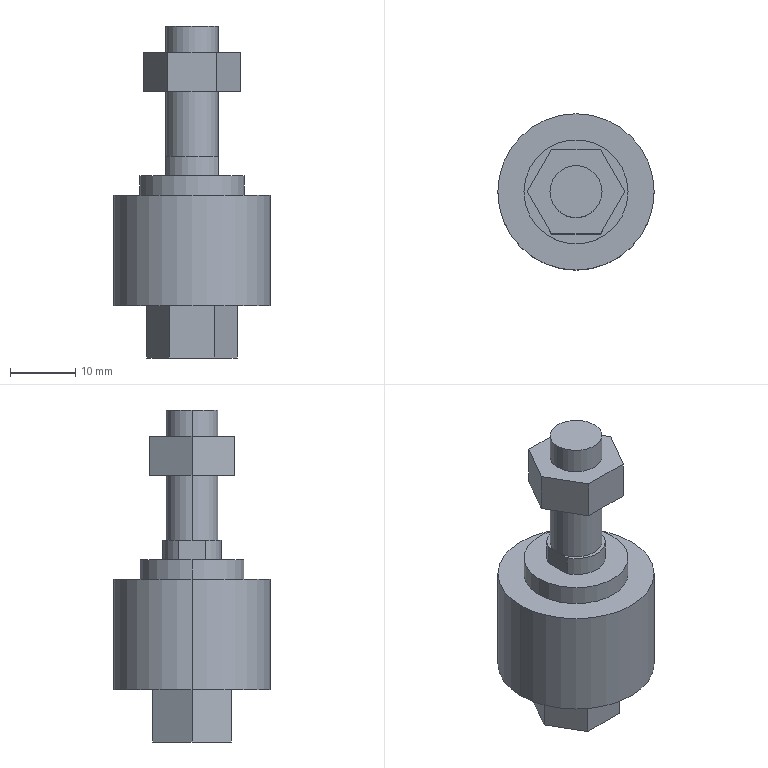Part | SolidWorks | features BaseBody 1 | 1 solid | 36 faces | box 24 x 24 x 51 mm | volume 10675 mm3 | plane 24 | cylinder 12 | commonest cylinder face diameters 8 x4 6.8 x2 9 x2 16 x2 24 x2
STEP:
#1=CARTESIAN_POINT('',(-3.4,0.,10.5));
#2=VERTEX_POINT('',#1);
#3=CARTESIAN_POINT('',(3.4,0.,10.5));
#4=VERTEX_POINT('',#3);
#5=CARTESIAN_POINT('',(0.,0.,10.5));
#6=DIRECTION('',(0.,0.,-1.));
#7=DIRECTION('',(-1.,0.,0.));
#8=AXIS2_PLACEMENT_3D('',#5,#6,#7);
#9=CIRCLE('',#8,3.4);
#10=EDGE_CURVE('',#2,#4,#9,.T.);
#11=ORIENTED_EDGE('',*,*,#10,.T.);
#12=CARTESIAN_POINT('',(0.,0.,10.5));
#13=DIRECTION('',(0.,0.,-1.));
#14=DIRECTION('',(-1.,0.,0.));
#15=AXIS2_PLACEMENT_3D('',#12,#13,#14);
#16=CIRCLE('',#15,3.4);
#17=EDGE_CURVE('',#4,#2,#16,.T.);
#18=ORIENTED_EDGE('',*,*,#17,.T.);
#19=EDGE_LOOP('',(#11,#18));
#20=FACE_OUTER_BOUND('',#19,.T.);
#21=CARTESIAN_POINT('',(0.,0.,10.5));
#22=DIRECTION('',(0.,0.,-1.));
#23=DIRECTION('',(0.,-1.,0.));
#24=AXIS2_PLACEMENT_3D('',#21,#22,#23);
#25=PLANE('',#24);
#26=ADVANCED_FACE('',(#20),#25,.T.);
#27=CARTESIAN_POINT('',(3.4,0.,0.));
#28=VERTEX_POINT('',#27);
#29=CARTESIAN_POINT('',(3.4,0.,10.5));
#30=DIRECTION('',(0.,0.,-1.));
#31=VECTOR('',#30,1000.);
#32=LINE('',#29,#31);
#33=EDGE_CURVE('',#4,#28,#32,.T.);
#34=ORIENTED_EDGE('',*,*,#33,.F.);
#35=ORIENTED_EDGE('',*,*,#10,.F.);
#36=CARTESIAN_POINT('',(-3.4,0.,0.));
#37=VERTEX_POINT('',#36);
#38=CARTESIAN_POINT('',(-3.4,0.,10.5));
#39=DIRECTION('',(0.,0.,-1.));
#40=VECTOR('',#39,1000.);
#41=LINE('',#38,#40);
#42=EDGE_CURVE('',#2,#37,#41,.T.);
#43=ORIENTED_EDGE('',*,*,#42,.T.);
#44=CARTESIAN_POINT('',(0.,0.,0.));
#45=DIRECTION('',(0.,0.,-1.));
#46=DIRECTION('',(-1.,0.,0.));
#47=AXIS2_PLACEMENT_3D('',#44,#45,#46);
#48=CIRCLE('',#47,3.4);
#49=EDGE_CURVE('',#37,#28,#48,.T.);
#50=ORIENTED_EDGE('',*,*,#49,.T.);
#51=EDGE_LOOP('',(#34,#35,#43,#50));
#52=FACE_OUTER_BOUND('',#51,.T.);
#53=CARTESIAN_POINT('',(0.,0.,10.5));
#54=DIRECTION('',(0.,0.,-1.));
#55=DIRECTION('',(-1.,0.,0.));
#56=AXIS2_PLACEMENT_3D('',#53,#54,#55);
#57=CYLINDRICAL_SURFACE('',#56,3.4);
#58=ADVANCED_FACE('',(#52),#57,.F.);
#59=CARTESIAN_POINT('',(4.,0.,51.));
#60=VERTEX_POINT('',#59);
#61=CARTESIAN_POINT('',(4.,0.,47.));
#62=VERTEX_POINT('',#61);
#63=CARTESIAN_POINT('',(4.,0.,0.));
#64=DIRECTION('',(0.,0.,-1.));
#65=VECTOR('',#64,1000.);
#66=LINE('',#63,#65);
#67=EDGE_CURVE('',#60,#62,#66,.T.);
#68=ORIENTED_EDGE('',*,*,#67,.F.);
#69=CARTESIAN_POINT('',(-4.,0.,51.));
#70=VERTEX_POINT('',#69);
#71=CARTESIAN_POINT('',(0.,0.,51.));
#72=DIRECTION('',(0.,0.,-1.));
#73=DIRECTION('',(-1.,0.,0.));
#74=AXIS2_PLACEMENT_3D('',#71,#72,#73);
#75=CIRCLE('',#74,4.);
#76=EDGE_CURVE('',#60,#70,#75,.T.);
#77=ORIENTED_EDGE('',*,*,#76,.T.);
#78=CARTESIAN_POINT('',(-4.,0.,47.));
#79=VERTEX_POINT('',#78);
#80=CARTESIAN_POINT('',(-4.,0.,0.));
#81=DIRECTION('',(0.,0.,-1.));
#82=VECTOR('',#81,1000.);
#83=LINE('',#80,#82);
#84=EDGE_CURVE('',#70,#79,#83,.T.);
#85=ORIENTED_EDGE('',*,*,#84,.T.);
#86=CARTESIAN_POINT('',(0.,0.,47.));
#87=DIRECTION('',(0.,0.,-1.));
#88=DIRECTION('',(1.,0.,0.));
#89=AXIS2_PLACEMENT_3D('',#86,#87,#88);
#90=CIRCLE('',#89,4.);
#91=EDGE_CURVE('',#62,#79,#90,.T.);
#92=ORIENTED_EDGE('',*,*,#91,.F.);
#93=EDGE_LOOP('',(#68,#77,#85,#92));
#94=FACE_OUTER_BOUND('',#93,.T.);
#95=CARTESIAN_POINT('',(0.,0.,0.));
#96=DIRECTION('',(0.,0.,-1.));
#97=DIRECTION('',(-1.,0.,0.));
#98=AXIS2_PLACEMENT_3D('',#95,#96,#97);
#99=CYLINDRICAL_SURFACE('',#98,4.);
#100=ADVANCED_FACE('',(#94),#99,.T.);
#101=CARTESIAN_POINT('',(0.,0.,51.));
#102=DIRECTION('',(0.,0.,-1.));
#103=DIRECTION('',(-1.,0.,0.));
#104=AXIS2_PLACEMENT_3D('',#101,#102,#103);
#105=CIRCLE('',#104,4.);
#106=EDGE_CURVE('',#70,#60,#105,.T.);
#107=ORIENTED_EDGE('',*,*,#106,.F.);
#108=ORIENTED_EDGE('',*,*,#76,.F.);
#109=EDGE_LOOP('',(#107,#108));
#110=FACE_OUTER_BOUND('',#109,.T.);
#111=CARTESIAN_POINT('',(0.,4.,51.));
#112=DIRECTION('',(0.,0.,1.));
#113=DIRECTION('',(1.,0.,0.));
#114=AXIS2_PLACEMENT_3D('',#111,#112,#113);
#115=PLANE('',#114);
#116=ADVANCED_FACE('',(#110),#115,.T.);
#117=CARTESIAN_POINT('',(0.,0.,47.));
#118=DIRECTION('',(0.,0.,-1.));
#119=DIRECTION('',(1.,0.,0.));
#120=AXIS2_PLACEMENT_3D('',#117,#118,#119);
#121=CIRCLE('',#120,4.);
#122=EDGE_CURVE('',#79,#62,#121,.T.);
#123=ORIENTED_EDGE('',*,*,#122,.T.);
#124=ORIENTED_EDGE('',*,*,#91,.T.);
#125=EDGE_LOOP('',(#123,#124));
#126=FACE_BOUND('',#125,.T.);
#127=CARTESIAN_POINT('',(-3.753,-6.5,47.));
#128=VERTEX_POINT('',#127);
#129=CARTESIAN_POINT('',(3.753,-6.5,47.));
#130=VERTEX_POINT('',#129);
#131=CARTESIAN_POINT('',(-3.753,-6.5,47.));
#132=DIRECTION('',(1.,0.,0.));
#133=VECTOR('',#132,1000.);
#134=LINE('',#131,#133);
#135=EDGE_CURVE('',#128,#130,#134,.T.);
#136=ORIENTED_EDGE('',*,*,#135,.T.);
#137=CARTESIAN_POINT('',(7.506,0.,47.));
#138=VERTEX_POINT('',#137);
#139=CARTESIAN_POINT('',(3.753,-6.5,47.));
#140=DIRECTION('',(0.5,0.866,0.));
#141=VECTOR('',#140,1000.);
#142=LINE('',#139,#141);
#143=EDGE_CURVE('',#130,#138,#142,.T.);
#144=ORIENTED_EDGE('',*,*,#143,.T.);
#145=CARTESIAN_POINT('',(3.753,6.5,47.));
#146=VERTEX_POINT('',#145);
#147=CARTESIAN_POINT('',(7.506,0.,47.));
#148=DIRECTION('',(-0.5,0.866,0.));
#149=VECTOR('',#148,1000.);
#150=LINE('',#147,#149);
#151=EDGE_CURVE('',#138,#146,#150,.T.);
#152=ORIENTED_EDGE('',*,*,#151,.T.);
#153=CARTESIAN_POINT('',(-3.753,6.5,47.));
#154=VERTEX_POINT('',#153);
#155=CARTESIAN_POINT('',(3.753,6.5,47.));
#156=DIRECTION('',(-1.,0.,0.));
#157=VECTOR('',#156,1000.);
#158=LINE('',#155,#157);
#159=EDGE_CURVE('',#146,#154,#158,.T.);
#160=ORIENTED_EDGE('',*,*,#159,.T.);
#161=CARTESIAN_POINT('',(-7.506,0.,47.));
#162=VERTEX_POINT('',#161);
#163=CARTESIAN_POINT('',(-3.753,6.5,47.));
#164=DIRECTION('',(-0.5,-0.866,0.));
#165=VECTOR('',#164,1000.);
#166=LINE('',#163,#165);
#167=EDGE_CURVE('',#154,#162,#166,.T.);
#168=ORIENTED_EDGE('',*,*,#167,.T.);
#169=CARTESIAN_POINT('',(-7.506,0.,47.));
#170=DIRECTION('',(0.5,-0.866,0.));
#171=VECTOR('',#170,1000.);
#172=LINE('',#169,#171);
#173=EDGE_CURVE('',#162,#128,#172,.T.);
#174=ORIENTED_EDGE('',*,*,#173,.T.);
#175=EDGE_LOOP('',(#136,#144,#152,#160,#168,#174));
#176=FACE_OUTER_BOUND('',#175,.T.);
#177=CARTESIAN_POINT('',(0.,0.,47.));
#178=DIRECTION('',(0.,0.,1.));
#179=DIRECTION('',(1.,0.,0.));
#180=AXIS2_PLACEMENT_3D('',#177,#178,#179);
#181=PLANE('',#180);
#182=ADVANCED_FACE('',(#126,#176),#181,.T.);
#183=CARTESIAN_POINT('',(-4.,0.,41.));
#184=VERTEX_POINT('',#183);
#185=CARTESIAN_POINT('',(4.,0.,41.));
#186=VERTEX_POINT('',#185);
#187=CARTESIAN_POINT('',(0.,0.,41.));
#188=DIRECTION('',(0.,0.,-1.));
#189=DIRECTION('',(1.,0.,0.));
#190=AXIS2_PLACEMENT_3D('',#187,#188,#189);
#191=CIRCLE('',#190,4.);
#192=EDGE_CURVE('',#184,#186,#191,.T.);
#193=ORIENTED_EDGE('',*,*,#192,.F.);
#194=CARTESIAN_POINT('',(0.,0.,41.));
#195=DIRECTION('',(0.,0.,-1.));
#196=DIRECTION('',(1.,0.,0.));
#197=AXIS2_PLACEMENT_3D('',#194,#195,#196);
#198=CIRCLE('',#197,4.);
#199=EDGE_CURVE('',#186,#184,#198,.T.);
#200=ORIENTED_EDGE('',*,*,#199,.F.);
#201=EDGE_LOOP('',(#193,#200));
#202=FACE_BOUND('',#201,.T.);
#203=CARTESIAN_POINT('',(-3.753,-6.5,41.));
#204=VERTEX_POINT('',#203);
#205=CARTESIAN_POINT('',(3.753,-6.5,41.));
#206=VERTEX_POINT('',#205);
#207=CARTESIAN_POINT('',(-3.753,-6.5,41.));
#208=DIRECTION('',(1.,0.,0.));
#209=VECTOR('',#208,1000.);
#210=LINE('',#207,#209);
#211=EDGE_CURVE('',#204,#206,#210,.T.);
#212=ORIENTED_EDGE('',*,*,#211,.F.);
#213=CARTESIAN_POINT('',(-7.506,0.,41.));
#214=VERTEX_POINT('',#213);
#215=CARTESIAN_POINT('',(-7.506,0.,41.));
#216=DIRECTION('',(0.5,-0.866,0.));
#217=VECTOR('',#216,1000.);
#218=LINE('',#215,#217);
#219=EDGE_CURVE('',#214,#204,#218,.T.);
#220=ORIENTED_EDGE('',*,*,#219,.F.);
#221=CARTESIAN_POINT('',(-3.753,6.5,41.));
#222=VERTEX_POINT('',#221);
#223=CARTESIAN_POINT('',(-3.753,6.5,41.));
#224=DIRECTION('',(-0.5,-0.866,0.));
#225=VECTOR('',#224,1000.);
#226=LINE('',#223,#225);
#227=EDGE_CURVE('',#222,#214,#226,.T.);
#228=ORIENTED_EDGE('',*,*,#227,.F.);
#229=CARTESIAN_POINT('',(3.753,6.5,41.));
#230=VERTEX_POINT('',#229);
#231=CARTESIAN_POINT('',(3.753,6.5,41.));
#232=DIRECTION('',(-1.,0.,0.));
#233=VECTOR('',#232,1000.);
#234=LINE('',#231,#233);
#235=EDGE_CURVE('',#230,#222,#234,.T.);
#236=ORIENTED_EDGE('',*,*,#235,.F.);
#237=CARTESIAN_POINT('',(7.506,0.,41.));
#238=VERTEX_POINT('',#237);
#239=CARTESIAN_POINT('',(7.506,0.,41.));
#240=DIRECTION('',(-0.5,0.866,0.));
#241=VECTOR('',#240,1000.);
#242=LINE('',#239,#241);
#243=EDGE_CURVE('',#238,#230,#242,.T.);
#244=ORIENTED_EDGE('',*,*,#243,.F.);
#245=CARTESIAN_POINT('',(3.753,-6.5,41.));
#246=DIRECTION('',(0.5,0.866,0.));
#247=VECTOR('',#246,1000.);
#248=LINE('',#245,#247);
#249=EDGE_CURVE('',#206,#238,#248,.T.);
#250=ORIENTED_EDGE('',*,*,#249,.F.);
#251=EDGE_LOOP('',(#212,#220,#228,#236,#244,#250));
#252=FACE_OUTER_BOUND('',#251,.T.);
#253=CARTESIAN_POINT('',(0.,0.,41.));
#254=DIRECTION('',(0.,0.,1.));
#255=DIRECTION('',(1.,0.,0.));
#256=AXIS2_PLACEMENT_3D('',#253,#254,#255);
#257=PLANE('',#256);
#258=ADVANCED_FACE('',(#202,#252),#257,.F.);
#259=ORIENTED_EDGE('',*,*,#143,.F.);
#260=CARTESIAN_POINT('',(3.753,-6.5,41.));
#261=DIRECTION('',(0.,0.,1.));
#262=VECTOR('',#261,1000.);
#263=LINE('',#260,#262);
#264=EDGE_CURVE('',#206,#130,#263,.T.);
#265=ORIENTED_EDGE('',*,*,#264,.F.);
#266=ORIENTED_EDGE('',*,*,#249,.T.);
#267=CARTESIAN_POINT('',(7.506,0.,41.));
#268=DIRECTION('',(0.,0.,1.));
#269=VECTOR('',#268,1000.);
#270=LINE('',#267,#269);
#271=EDGE_CURVE('',#238,#138,#270,.T.);
#272=ORIENTED_EDGE('',*,*,#271,.T.);
#273=EDGE_LOOP('',(#259,#265,#266,#272));
#274=FACE_OUTER_BOUND('',#273,.T.);
#275=CARTESIAN_POINT('',(3.753,-6.5,41.));
#276=DIRECTION('',(0.866,-0.5,0.));
#277=DIRECTION('',(0.,0.,-1.));
#278=AXIS2_PLACEMENT_3D('',#275,#276,#277);
#279=PLANE('',#278);
#280=ADVANCED_FACE('',(#274),#279,.T.);
#281=ORIENTED_EDGE('',*,*,#151,.F.);
#282=ORIENTED_EDGE('',*,*,#271,.F.);
#283=ORIENTED_EDGE('',*,*,#243,.T.);
#284=CARTESIAN_POINT('',(3.753,6.5,41.));
#285=DIRECTION('',(0.,0.,1.));
#286=VECTOR('',#285,1000.);
#287=LINE('',#284,#286);
#288=EDGE_CURVE('',#230,#146,#287,.T.);
#289=ORIENTED_EDGE('',*,*,#288,.T.);
#290=EDGE_LOOP('',(#281,#282,#283,#289));
#291=FACE_OUTER_BOUND('',#290,.T.);
#292=CARTESIAN_POINT('',(7.506,0.,41.));
#293=DIRECTION('',(0.866,0.5,0.));
#294=DIRECTION('',(0.,0.,-1.));
#295=AXIS2_PLACEMENT_3D('',#292,#293,#294);
#296=PLANE('',#295);
#297=ADVANCED_FACE('',(#291),#296,.T.);
#298=ORIENTED_EDGE('',*,*,#159,.F.);
#299=ORIENTED_EDGE('',*,*,#288,.F.);
#300=ORIENTED_EDGE('',*,*,#235,.T.);
#301=CARTESIAN_POINT('',(-3.753,6.5,41.));
#302=DIRECTION('',(0.,0.,1.));
#303=VECTOR('',#302,1000.);
#304=LINE('',#301,#303);
#305=EDGE_CURVE('',#222,#154,#304,.T.);
#306=ORIENTED_EDGE('',*,*,#305,.T.);
#307=EDGE_LOOP('',(#298,#299,#300,#306));
#308=FACE_OUTER_BOUND('',#307,.T.);
#309=CARTESIAN_POINT('',(3.753,6.5,41.));
#310=DIRECTION('',(0.,1.,0.));
#311=DIRECTION('',(1.,0.,0.));
#312=AXIS2_PLACEMENT_3D('',#309,#310,#311);
#313=PLANE('',#312);
#314=ADVANCED_FACE('',(#308),#313,.T.);
#315=ORIENTED_EDGE('',*,*,#167,.F.);
#316=ORIENTED_EDGE('',*,*,#305,.F.);
#317=ORIENTED_EDGE('',*,*,#227,.T.);
#318=CARTESIAN_POINT('',(-7.506,0.,41.));
#319=DIRECTION('',(0.,0.,1.));
#320=VECTOR('',#319,1000.);
#321=LINE('',#318,#320);
#322=EDGE_CURVE('',#214,#162,#321,.T.);
#323=ORIENTED_EDGE('',*,*,#322,.T.);
#324=EDGE_LOOP('',(#315,#316,#317,#323));
#325=FACE_OUTER_BOUND('',#324,.T.);
#326=CARTESIAN_POINT('',(-3.753,6.5,41.));
#327=DIRECTION('',(-0.866,0.5,0.));
#328=DIRECTION('',(0.,0.,1.));
#329=AXIS2_PLACEMENT_3D('',#326,#327,#328);
#330=PLANE('',#329);
#331=ADVANCED_FACE('',(#325),#330,.T.);
#332=ORIENTED_EDGE('',*,*,#173,.F.);
#333=ORIENTED_EDGE('',*,*,#322,.F.);
#334=ORIENTED_EDGE('',*,*,#219,.T.);
#335=CARTESIAN_POINT('',(-3.753,-6.5,41.));
#336=DIRECTION('',(0.,0.,1.));
#337=VECTOR('',#336,1000.);
#338=LINE('',#335,#337);
#339=EDGE_CURVE('',#204,#128,#338,.T.);
#340=ORIENTED_EDGE('',*,*,#339,.T.);
#341=EDGE_LOOP('',(#332,#333,#334,#340));
#342=FACE_OUTER_BOUND('',#341,.T.);
#343=CARTESIAN_POINT('',(-7.506,0.,41.));
#344=DIRECTION('',(-0.866,-0.5,0.));
#345=DIRECTION('',(-0.5,0.866,0.));
#346=AXIS2_PLACEMENT_3D('',#343,#344,#345);
#347=PLANE('',#346);
#348=ADVANCED_FACE('',(#342),#347,.T.);
#349=ORIENTED_EDGE('',*,*,#135,.F.);
#350=ORIENTED_EDGE('',*,*,#339,.F.);
#351=ORIENTED_EDGE('',*,*,#211,.T.);
#352=ORIENTED_EDGE('',*,*,#264,.T.);
#353=EDGE_LOOP('',(#349,#350,#351,#352));
#354=FACE_OUTER_BOUND('',#353,.T.);
#355=CARTESIAN_POINT('',(-3.753,-6.5,41.));
#356=DIRECTION('',(0.,-1.,0.));
#357=DIRECTION('',(0.,0.,-1.));
#358=AXIS2_PLACEMENT_3D('',#355,#356,#357);
#359=PLANE('',#358);
#360=ADVANCED_FACE('',(#354),#359,.T.);
#361=CARTESIAN_POINT('',(-4.,-2.062,28.));
#362=VERTEX_POINT('',#361);
#363=CARTESIAN_POINT('',(-4.,2.062,28.));
#364=VERTEX_POINT('',#363);
#365=CARTESIAN_POINT('',(-4.,-4.5,28.));
#366=DIRECTION('',(0.,1.,0.));
#367=VECTOR('',#366,1000.);
#368=LINE('',#365,#367);
#369=EDGE_CURVE('',#362,#364,#368,.T.);
#370=ORIENTED_EDGE('',*,*,#369,.F.);
#371=CARTESIAN_POINT('',(-4.,-2.062,31.));
#372=VERTEX_POINT('',#371);
#373=CARTESIAN_POINT('',(-4.,-2.062,0.));
#374=DIRECTION('',(0.,0.,-1.));
#375=VECTOR('',#374,1000.);
#376=LINE('',#373,#375);
#377=EDGE_CURVE('',#372,#362,#376,.T.);
#378=ORIENTED_EDGE('',*,*,#377,.F.);
#379=CARTESIAN_POINT('',(-4.,0.,31.));
#380=VERTEX_POINT('',#379);
#381=CARTESIAN_POINT('',(-4.,-4.5,31.));
#382=DIRECTION('',(0.,-1.,0.));
#383=VECTOR('',#382,1000.);
#384=LINE('',#381,#383);
#385=EDGE_CURVE('',#380,#372,#384,.T.);
#386=ORIENTED_EDGE('',*,*,#385,.F.);
#387=CARTESIAN_POINT('',(-4.,2.062,31.));
#388=VERTEX_POINT('',#387);
#389=CARTESIAN_POINT('',(-4.,-4.5,31.));
#390=DIRECTION('',(0.,-1.,0.));
#391=VECTOR('',#390,1000.);
#392=LINE('',#389,#391);
#393=EDGE_CURVE('',#388,#380,#392,.T.);
#394=ORIENTED_EDGE('',*,*,#393,.F.);
#395=CARTESIAN_POINT('',(-4.,2.062,0.));
#396=DIRECTION('',(0.,0.,1.));
#397=VECTOR('',#396,1000.);
#398=LINE('',#395,#397);
#399=EDGE_CURVE('',#364,#388,#398,.T.);
#400=ORIENTED_EDGE('',*,*,#399,.F.);
#401=EDGE_LOOP('',(#370,#378,#386,#394,#400));
#402=FACE_OUTER_BOUND('',#401,.T.);
#403=CARTESIAN_POINT('',(-4.,-4.5,-6.281));
#404=DIRECTION('',(-1.,0.,0.));
#405=DIRECTION('',(0.,0.,1.));
#406=AXIS2_PLACEMENT_3D('',#403,#404,#405);
#407=PLANE('',#406);
#408=ADVANCED_FACE('',(#402),#407,.T.);
#409=CARTESIAN_POINT('',(4.,2.062,28.));
#410=VERTEX_POINT('',#409);
#411=CARTESIAN_POINT('',(4.,-2.062,28.));
#412=VERTEX_POINT('',#411);
#413=CARTESIAN_POINT('',(4.,-4.5,28.));
#414=DIRECTION('',(0.,-1.,0.));
#415=VECTOR('',#414,1000.);
#416=LINE('',#413,#415);
#417=EDGE_CURVE('',#410,#412,#416,.T.);
#418=ORIENTED_EDGE('',*,*,#417,.F.);
#419=CARTESIAN_POINT('',(4.,2.062,31.));
#420=VERTEX_POINT('',#419);
#421=CARTESIAN_POINT('',(4.,2.062,0.));
#422=DIRECTION('',(0.,0.,-1.));
#423=VECTOR('',#422,1000.);
#424=LINE('',#421,#423);
#425=EDGE_CURVE('',#420,#410,#424,.T.);
#426=ORIENTED_EDGE('',*,*,#425,.F.);
#427=CARTESIAN_POINT('',(4.,0.,31.));
#428=VERTEX_POINT('',#427);
#429=CARTESIAN_POINT('',(4.,-4.5,31.));
#430=DIRECTION('',(0.,1.,0.));
#431=VECTOR('',#430,1000.);
#432=LINE('',#429,#431);
#433=EDGE_CURVE('',#428,#420,#432,.T.);
#434=ORIENTED_EDGE('',*,*,#433,.F.);
#435=CARTESIAN_POINT('',(4.,-2.062,31.));
#436=VERTEX_POINT('',#435);
#437=CARTESIAN_POINT('',(4.,-4.5,31.));
#438=DIRECTION('',(0.,1.,0.));
#439=VECTOR('',#438,1000.);
#440=LINE('',#437,#439);
#441=EDGE_CURVE('',#436,#428,#440,.T.);
#442=ORIENTED_EDGE('',*,*,#441,.F.);
#443=CARTESIAN_POINT('',(4.,-2.062,0.));
#444=DIRECTION('',(0.,0.,1.));
#445=VECTOR('',#444,1000.);
#446=LINE('',#443,#445);
#447=EDGE_CURVE('',#412,#436,#446,.T.);
#448=ORIENTED_EDGE('',*,*,#447,.F.);
#449=EDGE_LOOP('',(#418,#426,#434,#442,#448));
#450=FACE_OUTER_BOUND('',#449,.T.);
#451=CARTESIAN_POINT('',(4.,-4.5,-6.281));
#452=DIRECTION('',(1.,0.,0.));
#453=DIRECTION('',(0.,1.,0.));
#454=AXIS2_PLACEMENT_3D('',#451,#452,#453);
#455=PLANE('',#454);
#456=ADVANCED_FACE('',(#450),#455,.T.);
#457=CARTESIAN_POINT('',(0.,0.,28.));
#458=DIRECTION('',(0.,0.,-1.));
#459=DIRECTION('',(-1.,0.,0.));
#460=AXIS2_PLACEMENT_3D('',#457,#458,#459);
#461=CIRCLE('',#460,4.5);
#462=EDGE_CURVE('',#364,#410,#461,.T.);
#463=ORIENTED_EDGE('',*,*,#462,.T.);
#464=ORIENTED_EDGE('',*,*,#417,.T.);
#465=CARTESIAN_POINT('',(0.,0.,28.));
#466=DIRECTION('',(0.,0.,-1.));
#467=DIRECTION('',(-1.,0.,0.));
#468=AXIS2_PLACEMENT_3D('',#465,#466,#467);
#469=CIRCLE('',#468,4.5);
#470=EDGE_CURVE('',#412,#362,#469,.T.);
#471=ORIENTED_EDGE('',*,*,#470,.T.);
#472=ORIENTED_EDGE('',*,*,#369,.T.);
#473=EDGE_LOOP('',(#463,#464,#471,#472));
#474=FACE_BOUND('',#473,.T.);
#475=CARTESIAN_POINT('',(-8.,0.,28.));
#476=VERTEX_POINT('',#475);
#477=CARTESIAN_POINT('',(8.,0.,28.));
#478=VERTEX_POINT('',#477);
#479=CARTESIAN_POINT('',(0.,0.,28.));
#480=DIRECTION('',(0.,0.,-1.));
#481=DIRECTION('',(-1.,0.,0.));
#482=AXIS2_PLACEMENT_3D('',#479,#480,#481);
#483=CIRCLE('',#482,8.);
#484=EDGE_CURVE('',#476,#478,#483,.T.);
#485=ORIENTED_EDGE('',*,*,#484,.F.);
#486=CARTESIAN_POINT('',(0.,0.,28.));
#487=DIRECTION('',(0.,0.,-1.));
#488=DIRECTION('',(-1.,0.,0.));
#489=AXIS2_PLACEMENT_3D('',#486,#487,#488);
#490=CIRCLE('',#489,8.);
#491=EDGE_CURVE('',#478,#476,#490,.T.);
#492=ORIENTED_EDGE('',*,*,#491,.F.);
#493=EDGE_LOOP('',(#485,#492));
#494=FACE_OUTER_BOUND('',#493,.T.);
#495=CARTESIAN_POINT('',(0.,8.,28.));
#496=DIRECTION('',(0.,0.,1.));
#497=DIRECTION('',(1.,0.,0.));
#498=AXIS2_PLACEMENT_3D('',#495,#496,#497);
#499=PLANE('',#498);
#500=ADVANCED_FACE('',(#474,#494),#499,.T.);
#501=CARTESIAN_POINT('',(8.,0.,25.));
#502=VERTEX_POINT('',#501);
#503=CARTESIAN_POINT('',(8.,0.,0.));
#504=DIRECTION('',(0.,0.,-1.));
#505=VECTOR('',#504,1000.);
#506=LINE('',#503,#505);
#507=EDGE_CURVE('',#478,#502,#506,.T.);
#508=ORIENTED_EDGE('',*,*,#507,.F.);
#509=ORIENTED_EDGE('',*,*,#491,.T.);
#510=CARTESIAN_POINT('',(-8.,0.,25.));
#511=VERTEX_POINT('',#510);
#512=CARTESIAN_POINT('',(-8.,0.,0.));
#513=DIRECTION('',(0.,0.,-1.));
#514=VECTOR('',#513,1000.);
#515=LINE('',#512,#514);
#516=EDGE_CURVE('',#476,#511,#515,.T.);
#517=ORIENTED_EDGE('',*,*,#516,.T.);
#518=CARTESIAN_POINT('',(0.,0.,25.));
#519=DIRECTION('',(0.,0.,-1.));
#520=DIRECTION('',(-1.,0.,0.));
#521=AXIS2_PLACEMENT_3D('',#518,#519,#520);
#522=CIRCLE('',#521,8.);
#523=EDGE_CURVE('',#502,#511,#522,.T.);
#524=ORIENTED_EDGE('',*,*,#523,.F.);
#525=EDGE_LOOP('',(#508,#509,#517,#524));
#526=FACE_OUTER_BOUND('',#525,.T.);
#527=CARTESIAN_POINT('',(0.,0.,0.));
#528=DIRECTION('',(0.,0.,-1.));
#529=DIRECTION('',(-1.,0.,0.));
#530=AXIS2_PLACEMENT_3D('',#527,#528,#529);
#531=CYLINDRICAL_SURFACE('',#530,8.);
#532=ADVANCED_FACE('',(#526),#531,.T.);
#533=CARTESIAN_POINT('',(0.,0.,25.));
#534=DIRECTION('',(0.,0.,-1.));
#535=DIRECTION('',(-1.,0.,0.));
#536=AXIS2_PLACEMENT_3D('',#533,#534,#535);
#537=CIRCLE('',#536,8.);
#538=EDGE_CURVE('',#511,#502,#537,.T.);
#539=ORIENTED_EDGE('',*,*,#538,.T.);
#540=ORIENTED_EDGE('',*,*,#523,.T.);
#541=EDGE_LOOP('',(#539,#540));
#542=FACE_BOUND('',#541,.T.);
#543=CARTESIAN_POINT('',(-12.,0.,25.));
#544=VERTEX_POINT('',#543);
#545=CARTESIAN_POINT('',(12.,0.,25.));
#546=VERTEX_POINT('',#545);
#547=CARTESIAN_POINT('',(0.,0.,25.));
#548=DIRECTION('',(0.,0.,-1.));
#549=DIRECTION('',(-1.,0.,0.));
#550=AXIS2_PLACEMENT_3D('',#547,#548,#549);
#551=CIRCLE('',#550,12.);
#552=EDGE_CURVE('',#544,#546,#551,.T.);
#553=ORIENTED_EDGE('',*,*,#552,.F.);
#554=CARTESIAN_POINT('',(0.,0.,25.));
#555=DIRECTION('',(0.,0.,-1.));
#556=DIRECTION('',(-1.,0.,0.));
#557=AXIS2_PLACEMENT_3D('',#554,#555,#556);
#558=CIRCLE('',#557,12.);
#559=EDGE_CURVE('',#546,#544,#558,.T.);
#560=ORIENTED_EDGE('',*,*,#559,.F.);
#561=EDGE_LOOP('',(#553,#560));
#562=FACE_OUTER_BOUND('',#561,.T.);
#563=CARTESIAN_POINT('',(0.,12.,25.));
#564=DIRECTION('',(0.,0.,1.));
#565=DIRECTION('',(1.,0.,0.));
#566=AXIS2_PLACEMENT_3D('',#563,#564,#565);
#567=PLANE('',#566);
#568=ADVANCED_FACE('',(#542,#562),#567,.T.);
#569=CARTESIAN_POINT('',(12.,0.,8.));
#570=VERTEX_POINT('',#569);
#571=CARTESIAN_POINT('',(12.,0.,0.));
#572=DIRECTION('',(0.,0.,-1.));
#573=VECTOR('',#572,1000.);
#574=LINE('',#571,#573);
#575=EDGE_CURVE('',#546,#570,#574,.T.);
#576=ORIENTED_EDGE('',*,*,#575,.F.);
#577=ORIENTED_EDGE('',*,*,#559,.T.);
#578=CARTESIAN_POINT('',(-12.,0.,8.));
#579=VERTEX_POINT('',#578);
#580=CARTESIAN_POINT('',(-12.,0.,0.));
#581=DIRECTION('',(0.,0.,-1.));
#582=VECTOR('',#581,1000.);
#583=LINE('',#580,#582);
#584=EDGE_CURVE('',#544,#579,#583,.T.);
#585=ORIENTED_EDGE('',*,*,#584,.T.);
#586=CARTESIAN_POINT('',(0.,0.,8.));
#587=DIRECTION('',(0.,0.,-1.));
#588=DIRECTION('',(-1.,0.,0.));
#589=AXIS2_PLACEMENT_3D('',#586,#587,#588);
#590=CIRCLE('',#589,12.);
#591=EDGE_CURVE('',#570,#579,#590,.T.);
#592=ORIENTED_EDGE('',*,*,#591,.F.);
#593=EDGE_LOOP('',(#576,#577,#585,#592));
#594=FACE_OUTER_BOUND('',#593,.T.);
#595=CARTESIAN_POINT('',(0.,0.,0.));
#596=DIRECTION('',(0.,0.,-1.));
#597=DIRECTION('',(-1.,0.,0.));
#598=AXIS2_PLACEMENT_3D('',#595,#596,#597);
#599=CYLINDRICAL_SURFACE('',#598,12.);
#600=ADVANCED_FACE('',(#594),#599,.T.);
#601=CARTESIAN_POINT('',(-3.464,-6.,8.));
#602=VERTEX_POINT('',#601);
#603=CARTESIAN_POINT('',(3.464,-6.,8.));
#604=VERTEX_POINT('',#603);
#605=CARTESIAN_POINT('',(-3.464,-6.,8.));
#606=DIRECTION('',(1.,0.,0.));
#607=VECTOR('',#606,1000.);
#608=LINE('',#605,#607);
#609=EDGE_CURVE('',#602,#604,#608,.T.);
#610=ORIENTED_EDGE('',*,*,#609,.T.);
#611=CARTESIAN_POINT('',(6.928,0.,8.));
#612=VERTEX_POINT('',#611);
#613=CARTESIAN_POINT('',(3.464,-6.,8.));
#614=DIRECTION('',(0.5,0.866,0.));
#615=VECTOR('',#614,1000.);
#616=LINE('',#613,#615);
#617=EDGE_CURVE('',#604,#612,#616,.T.);
#618=ORIENTED_EDGE('',*,*,#617,.T.);
#619=CARTESIAN_POINT('',(3.464,6.,8.));
#620=VERTEX_POINT('',#619);
#621=CARTESIAN_POINT('',(6.928,0.,8.));
#622=DIRECTION('',(-0.5,0.866,0.));
#623=VECTOR('',#622,1000.);
#624=LINE('',#621,#623);
#625=EDGE_CURVE('',#612,#620,#624,.T.);
#626=ORIENTED_EDGE('',*,*,#625,.T.);
#627=CARTESIAN_POINT('',(-3.464,6.,8.));
#628=VERTEX_POINT('',#627);
#629=CARTESIAN_POINT('',(3.464,6.,8.));
#630=DIRECTION('',(-1.,0.,0.));
#631=VECTOR('',#630,1000.);
#632=LINE('',#629,#631);
#633=EDGE_CURVE('',#620,#628,#632,.T.);
#634=ORIENTED_EDGE('',*,*,#633,.T.);
#635=CARTESIAN_POINT('',(-6.928,0.,8.));
#636=VERTEX_POINT('',#635);
#637=CARTESIAN_POINT('',(-3.464,6.,8.));
#638=DIRECTION('',(-0.5,-0.866,0.));
#639=VECTOR('',#638,1000.);
#640=LINE('',#637,#639);
#641=EDGE_CURVE('',#628,#636,#640,.T.);
#642=ORIENTED_EDGE('',*,*,#641,.T.);
#643=CARTESIAN_POINT('',(-6.928,0.,8.));
#644=DIRECTION('',(0.5,-0.866,0.));
#645=VECTOR('',#644,1000.);
#646=LINE('',#643,#645);
#647=EDGE_CURVE('',#636,#602,#646,.T.);
#648=ORIENTED_EDGE('',*,*,#647,.T.);
#649=EDGE_LOOP('',(#610,#618,#626,#634,#642,#648));
#650=FACE_BOUND('',#649,.T.);
#651=CARTESIAN_POINT('',(0.,0.,8.));
#652=DIRECTION('',(0.,0.,-1.));
#653=DIRECTION('',(-1.,0.,0.));
#654=AXIS2_PLACEMENT_3D('',#651,#652,#653);
#655=CIRCLE('',#654,12.);
#656=EDGE_CURVE('',#579,#570,#655,.T.);
#657=ORIENTED_EDGE('',*,*,#656,.T.);
#658=ORIENTED_EDGE('',*,*,#591,.T.);
#659=EDGE_LOOP('',(#657,#658));
#660=FACE_OUTER_BOUND('',#659,.T.);
#661=CARTESIAN_POINT('',(0.,0.,8.));
#662=DIRECTION('',(0.,0.,-1.));
#663=DIRECTION('',(0.,-1.,0.));
#664=AXIS2_PLACEMENT_3D('',#661,#662,#663);
#665=PLANE('',#664);
#666=ADVANCED_FACE('',(#650,#660),#665,.T.);
#667=ORIENTED_EDGE('',*,*,#49,.F.);
#668=CARTESIAN_POINT('',(0.,0.,0.));
#669=DIRECTION('',(0.,0.,-1.));
#670=DIRECTION('',(-1.,0.,0.));
#671=AXIS2_PLACEMENT_3D('',#668,#669,#670);
#672=CIRCLE('',#671,3.4);
#673=EDGE_CURVE('',#28,#37,#672,.T.);
#674=ORIENTED_EDGE('',*,*,#673,.F.);
#675=EDGE_LOOP('',(#667,#674));
#676=FACE_BOUND('',#675,.T.);
#677=CARTESIAN_POINT('',(-3.464,-6.,0.));
#678=VERTEX_POINT('',#677);
#679=CARTESIAN_POINT('',(3.464,-6.,0.));
#680=VERTEX_POINT('',#679);
#681=CARTESIAN_POINT('',(-3.464,-6.,0.));
#682=DIRECTION('',(1.,0.,0.));
#683=VECTOR('',#682,1000.);
#684=LINE('',#681,#683);
#685=EDGE_CURVE('',#678,#680,#684,.T.);
#686=ORIENTED_EDGE('',*,*,#685,.F.);
#687=CARTESIAN_POINT('',(-6.928,0.,0.));
#688=VERTEX_POINT('',#687);
#689=CARTESIAN_POINT('',(-6.928,0.,0.));
#690=DIRECTION('',(0.5,-0.866,0.));
#691=VECTOR('',#690,1000.);
#692=LINE('',#689,#691);
#693=EDGE_CURVE('',#688,#678,#692,.T.);
#694=ORIENTED_EDGE('',*,*,#693,.F.);
#695=CARTESIAN_POINT('',(-3.464,6.,0.));
#696=VERTEX_POINT('',#695);
#697=CARTESIAN_POINT('',(-3.464,6.,0.));
#698=DIRECTION('',(-0.5,-0.866,0.));
#699=VECTOR('',#698,1000.);
#700=LINE('',#697,#699);
#701=EDGE_CURVE('',#696,#688,#700,.T.);
#702=ORIENTED_EDGE('',*,*,#701,.F.);
#703=CARTESIAN_POINT('',(3.464,6.,0.));
#704=VERTEX_POINT('',#703);
#705=CARTESIAN_POINT('',(3.464,6.,0.));
#706=DIRECTION('',(-1.,0.,0.));
#707=VECTOR('',#706,1000.);
#708=LINE('',#705,#707);
#709=EDGE_CURVE('',#704,#696,#708,.T.);
#710=ORIENTED_EDGE('',*,*,#709,.F.);
#711=CARTESIAN_POINT('',(6.928,0.,0.));
#712=VERTEX_POINT('',#711);
#713=CARTESIAN_POINT('',(6.928,0.,0.));
#714=DIRECTION('',(-0.5,0.866,0.));
#715=VECTOR('',#714,1000.);
#716=LINE('',#713,#715);
#717=EDGE_CURVE('',#712,#704,#716,.T.);
#718=ORIENTED_EDGE('',*,*,#717,.F.);
#719=CARTESIAN_POINT('',(3.464,-6.,0.));
#720=DIRECTION('',(0.5,0.866,0.));
#721=VECTOR('',#720,1000.);
#722=LINE('',#719,#721);
#723=EDGE_CURVE('',#680,#712,#722,.T.);
#724=ORIENTED_EDGE('',*,*,#723,.F.);
#725=EDGE_LOOP('',(#686,#694,#702,#710,#718,#724));
#726=FACE_OUTER_BOUND('',#725,.T.);
#727=CARTESIAN_POINT('',(0.,0.,0.));
#728=DIRECTION('',(0.,0.,1.));
#729=DIRECTION('',(1.,0.,0.));
#730=AXIS2_PLACEMENT_3D('',#727,#728,#729);
#731=PLANE('',#730);
#732=ADVANCED_FACE('',(#676,#726),#731,.F.);
#733=ORIENTED_EDGE('',*,*,#693,.T.);
#734=CARTESIAN_POINT('',(-3.464,-6.,8.));
#735=DIRECTION('',(0.,0.,-1.));
#736=VECTOR('',#735,1000.);
#737=LINE('',#734,#736);
#738=EDGE_CURVE('',#602,#678,#737,.T.);
#739=ORIENTED_EDGE('',*,*,#738,.F.);
#740=ORIENTED_EDGE('',*,*,#647,.F.);
#741=CARTESIAN_POINT('',(-6.928,0.,8.));
#742=DIRECTION('',(0.,0.,-1.));
#743=VECTOR('',#742,1000.);
#744=LINE('',#741,#743);
#745=EDGE_CURVE('',#636,#688,#744,.T.);
#746=ORIENTED_EDGE('',*,*,#745,.T.);
#747=EDGE_LOOP('',(#733,#739,#740,#746));
#748=FACE_OUTER_BOUND('',#747,.T.);
#749=CARTESIAN_POINT('',(-6.928,0.,8.));
#750=DIRECTION('',(0.866,0.5,0.));
#751=DIRECTION('',(0.,0.,-1.));
#752=AXIS2_PLACEMENT_3D('',#749,#750,#751);
#753=PLANE('',#752);
#754=ADVANCED_FACE('',(#748),#753,.F.);
#755=ORIENTED_EDGE('',*,*,#701,.T.);
#756=ORIENTED_EDGE('',*,*,#745,.F.);
#757=ORIENTED_EDGE('',*,*,#641,.F.);
#758=CARTESIAN_POINT('',(-3.464,6.,8.));
#759=DIRECTION('',(0.,0.,-1.));
#760=VECTOR('',#759,1000.);
#761=LINE('',#758,#760);
#762=EDGE_CURVE('',#628,#696,#761,.T.);
#763=ORIENTED_EDGE('',*,*,#762,.T.);
#764=EDGE_LOOP('',(#755,#756,#757,#763));
#765=FACE_OUTER_BOUND('',#764,.T.);
#766=CARTESIAN_POINT('',(-3.464,6.,8.));
#767=DIRECTION('',(0.866,-0.5,0.));
#768=DIRECTION('',(0.,0.,-1.));
#769=AXIS2_PLACEMENT_3D('',#766,#767,#768);
#770=PLANE('',#769);
#771=ADVANCED_FACE('',(#765),#770,.F.);
#772=ORIENTED_EDGE('',*,*,#709,.T.);
#773=ORIENTED_EDGE('',*,*,#762,.F.);
#774=ORIENTED_EDGE('',*,*,#633,.F.);
#775=CARTESIAN_POINT('',(3.464,6.,8.));
#776=DIRECTION('',(0.,0.,-1.));
#777=VECTOR('',#776,1000.);
#778=LINE('',#775,#777);
#779=EDGE_CURVE('',#620,#704,#778,.T.);
#780=ORIENTED_EDGE('',*,*,#779,.T.);
#781=EDGE_LOOP('',(#772,#773,#774,#780));
#782=FACE_OUTER_BOUND('',#781,.T.);
#783=CARTESIAN_POINT('',(3.464,6.,8.));
#784=DIRECTION('',(0.,-1.,0.));
#785=DIRECTION('',(0.,0.,-1.));
#786=AXIS2_PLACEMENT_3D('',#783,#784,#785);
#787=PLANE('',#786);
#788=ADVANCED_FACE('',(#782),#787,.F.);
#789=ORIENTED_EDGE('',*,*,#717,.T.);
#790=ORIENTED_EDGE('',*,*,#779,.F.);
#791=ORIENTED_EDGE('',*,*,#625,.F.);
#792=CARTESIAN_POINT('',(6.928,0.,8.));
#793=DIRECTION('',(0.,0.,-1.));
#794=VECTOR('',#793,1000.);
#795=LINE('',#792,#794);
#796=EDGE_CURVE('',#612,#712,#795,.T.);
#797=ORIENTED_EDGE('',*,*,#796,.T.);
#798=EDGE_LOOP('',(#789,#790,#791,#797));
#799=FACE_OUTER_BOUND('',#798,.T.);
#800=CARTESIAN_POINT('',(6.928,0.,8.));
#801=DIRECTION('',(-0.866,-0.5,0.));
#802=DIRECTION('',(-0.5,0.866,0.));
#803=AXIS2_PLACEMENT_3D('',#800,#801,#802);
#804=PLANE('',#803);
#805=ADVANCED_FACE('',(#799),#804,.F.);
#806=ORIENTED_EDGE('',*,*,#723,.T.);
#807=ORIENTED_EDGE('',*,*,#796,.F.);
#808=ORIENTED_EDGE('',*,*,#617,.F.);
#809=CARTESIAN_POINT('',(3.464,-6.,8.));
#810=DIRECTION('',(0.,0.,-1.));
#811=VECTOR('',#810,1000.);
#812=LINE('',#809,#811);
#813=EDGE_CURVE('',#604,#680,#812,.T.);
#814=ORIENTED_EDGE('',*,*,#813,.T.);
#815=EDGE_LOOP('',(#806,#807,#808,#814));
#816=FACE_OUTER_BOUND('',#815,.T.);
#817=CARTESIAN_POINT('',(3.464,-6.,8.));
#818=DIRECTION('',(-0.866,0.5,0.));
#819=DIRECTION('',(0.,0.,1.));
#820=AXIS2_PLACEMENT_3D('',#817,#818,#819);
#821=PLANE('',#820);
#822=ADVANCED_FACE('',(#816),#821,.F.);
#823=ORIENTED_EDGE('',*,*,#685,.T.);
#824=ORIENTED_EDGE('',*,*,#813,.F.);
#825=ORIENTED_EDGE('',*,*,#609,.F.);
#826=ORIENTED_EDGE('',*,*,#738,.T.);
#827=EDGE_LOOP('',(#823,#824,#825,#826));
#828=FACE_OUTER_BOUND('',#827,.T.);
#829=CARTESIAN_POINT('',(-3.464,-6.,8.));
#830=DIRECTION('',(0.,1.,0.));
#831=DIRECTION('',(1.,0.,0.));
#832=AXIS2_PLACEMENT_3D('',#829,#830,#831);
#833=PLANE('',#832);
#834=ADVANCED_FACE('',(#828),#833,.F.);
#835=CARTESIAN_POINT('',(0.,0.,31.));
#836=DIRECTION('',(0.,0.,-1.));
#837=DIRECTION('',(-1.,0.,0.));
#838=AXIS2_PLACEMENT_3D('',#835,#836,#837);
#839=CIRCLE('',#838,4.);
#840=EDGE_CURVE('',#428,#380,#839,.T.);
#841=ORIENTED_EDGE('',*,*,#840,.T.);
#842=ORIENTED_EDGE('',*,*,#385,.T.);
#843=CARTESIAN_POINT('',(0.,0.,31.));
#844=DIRECTION('',(0.,0.,-1.));
#845=DIRECTION('',(-1.,0.,0.));
#846=AXIS2_PLACEMENT_3D('',#843,#844,#845);
#847=CIRCLE('',#846,4.5);
#848=EDGE_CURVE('',#436,#372,#847,.T.);
#849=ORIENTED_EDGE('',*,*,#848,.F.);
#850=ORIENTED_EDGE('',*,*,#441,.T.);
#851=EDGE_LOOP('',(#841,#842,#849,#850));
#852=FACE_OUTER_BOUND('',#851,.T.);
#853=CARTESIAN_POINT('',(0.,4.5,31.));
#854=DIRECTION('',(0.,0.,1.));
#855=DIRECTION('',(1.,0.,0.));
#856=AXIS2_PLACEMENT_3D('',#853,#854,#855);
#857=PLANE('',#856);
#858=ADVANCED_FACE('',(#852),#857,.T.);
#859=CARTESIAN_POINT('',(0.,0.,31.));
#860=DIRECTION('',(0.,0.,-1.));
#861=DIRECTION('',(-1.,0.,0.));
#862=AXIS2_PLACEMENT_3D('',#859,#860,#861);
#863=CIRCLE('',#862,4.5);
#864=EDGE_CURVE('',#388,#420,#863,.T.);
#865=ORIENTED_EDGE('',*,*,#864,.F.);
#866=ORIENTED_EDGE('',*,*,#393,.T.);
#867=CARTESIAN_POINT('',(0.,0.,31.));
#868=DIRECTION('',(0.,0.,-1.));
#869=DIRECTION('',(-1.,0.,0.));
#870=AXIS2_PLACEMENT_3D('',#867,#868,#869);
#871=CIRCLE('',#870,4.);
#872=EDGE_CURVE('',#380,#428,#871,.T.);
#873=ORIENTED_EDGE('',*,*,#872,.T.);
#874=ORIENTED_EDGE('',*,*,#433,.T.);
#875=EDGE_LOOP('',(#865,#866,#873,#874));
#876=FACE_OUTER_BOUND('',#875,.T.);
#877=CARTESIAN_POINT('',(0.,4.5,31.));
#878=DIRECTION('',(0.,0.,1.));
#879=DIRECTION('',(1.,0.,0.));
#880=AXIS2_PLACEMENT_3D('',#877,#878,#879);
#881=PLANE('',#880);
#882=ADVANCED_FACE('',(#876),#881,.T.);
#883=ORIENTED_EDGE('',*,*,#848,.T.);
#884=ORIENTED_EDGE('',*,*,#377,.T.);
#885=ORIENTED_EDGE('',*,*,#470,.F.);
#886=ORIENTED_EDGE('',*,*,#447,.T.);
#887=EDGE_LOOP('',(#883,#884,#885,#886));
#888=FACE_OUTER_BOUND('',#887,.T.);
#889=CARTESIAN_POINT('',(0.,0.,0.));
#890=DIRECTION('',(0.,0.,-1.));
#891=DIRECTION('',(-1.,0.,0.));
#892=AXIS2_PLACEMENT_3D('',#889,#890,#891);
#893=CYLINDRICAL_SURFACE('',#892,4.5);
#894=ADVANCED_FACE('',(#888),#893,.T.);
#895=ORIENTED_EDGE('',*,*,#864,.T.);
#896=ORIENTED_EDGE('',*,*,#425,.T.);
#897=ORIENTED_EDGE('',*,*,#462,.F.);
#898=ORIENTED_EDGE('',*,*,#399,.T.);
#899=EDGE_LOOP('',(#895,#896,#897,#898));
#900=FACE_OUTER_BOUND('',#899,.T.);
#901=CARTESIAN_POINT('',(0.,0.,0.));
#902=DIRECTION('',(0.,0.,-1.));
#903=DIRECTION('',(-1.,0.,0.));
#904=AXIS2_PLACEMENT_3D('',#901,#902,#903);
#905=CYLINDRICAL_SURFACE('',#904,4.5);
#906=ADVANCED_FACE('',(#900),#905,.T.);
#907=CARTESIAN_POINT('',(4.,0.,0.));
#908=DIRECTION('',(0.,0.,-1.));
#909=VECTOR('',#908,1000.);
#910=LINE('',#907,#909);
#911=EDGE_CURVE('',#186,#428,#910,.T.);
#912=ORIENTED_EDGE('',*,*,#911,.F.);
#913=ORIENTED_EDGE('',*,*,#199,.T.);
#914=CARTESIAN_POINT('',(-4.,0.,0.));
#915=DIRECTION('',(0.,0.,-1.));
#916=VECTOR('',#915,1000.);
#917=LINE('',#914,#916);
#918=EDGE_CURVE('',#184,#380,#917,.T.);
#919=ORIENTED_EDGE('',*,*,#918,.T.);
#920=ORIENTED_EDGE('',*,*,#840,.F.);
#921=EDGE_LOOP('',(#912,#913,#919,#920));
#922=FACE_OUTER_BOUND('',#921,.T.);
#923=CARTESIAN_POINT('',(0.,0.,0.));
#924=DIRECTION('',(0.,0.,-1.));
#925=DIRECTION('',(-1.,0.,0.));
#926=AXIS2_PLACEMENT_3D('',#923,#924,#925);
#927=CYLINDRICAL_SURFACE('',#926,4.);
#928=ADVANCED_FACE('',(#922),#927,.T.);
#929=ORIENTED_EDGE('',*,*,#192,.T.);
#930=ORIENTED_EDGE('',*,*,#911,.T.);
#931=ORIENTED_EDGE('',*,*,#872,.F.);
#932=ORIENTED_EDGE('',*,*,#918,.F.);
#933=EDGE_LOOP('',(#929,#930,#931,#932));
#934=FACE_OUTER_BOUND('',#933,.T.);
#935=CARTESIAN_POINT('',(0.,0.,0.));
#936=DIRECTION('',(0.,0.,-1.));
#937=DIRECTION('',(-1.,0.,0.));
#938=AXIS2_PLACEMENT_3D('',#935,#936,#937);
#939=CYLINDRICAL_SURFACE('',#938,4.);
#940=ADVANCED_FACE('',(#934),#939,.T.);
#941=ORIENTED_EDGE('',*,*,#552,.T.);
#942=ORIENTED_EDGE('',*,*,#575,.T.);
#943=ORIENTED_EDGE('',*,*,#656,.F.);
#944=ORIENTED_EDGE('',*,*,#584,.F.);
#945=EDGE_LOOP('',(#941,#942,#943,#944));
#946=FACE_OUTER_BOUND('',#945,.T.);
#947=CARTESIAN_POINT('',(0.,0.,0.));
#948=DIRECTION('',(0.,0.,-1.));
#949=DIRECTION('',(-1.,0.,0.));
#950=AXIS2_PLACEMENT_3D('',#947,#948,#949);
#951=CYLINDRICAL_SURFACE('',#950,12.);
#952=ADVANCED_FACE('',(#946),#951,.T.);
#953=ORIENTED_EDGE('',*,*,#484,.T.);
#954=ORIENTED_EDGE('',*,*,#507,.T.);
#955=ORIENTED_EDGE('',*,*,#538,.F.);
#956=ORIENTED_EDGE('',*,*,#516,.F.);
#957=EDGE_LOOP('',(#953,#954,#955,#956));
#958=FACE_OUTER_BOUND('',#957,.T.);
#959=CARTESIAN_POINT('',(0.,0.,0.));
#960=DIRECTION('',(0.,0.,-1.));
#961=DIRECTION('',(-1.,0.,0.));
#962=AXIS2_PLACEMENT_3D('',#959,#960,#961);
#963=CYLINDRICAL_SURFACE('',#962,8.);
#964=ADVANCED_FACE('',(#958),#963,.T.);
#965=ORIENTED_EDGE('',*,*,#106,.T.);
#966=ORIENTED_EDGE('',*,*,#67,.T.);
#967=ORIENTED_EDGE('',*,*,#122,.F.);
#968=ORIENTED_EDGE('',*,*,#84,.F.);
#969=EDGE_LOOP('',(#965,#966,#967,#968));
#970=FACE_OUTER_BOUND('',#969,.T.);
#971=CARTESIAN_POINT('',(0.,0.,0.));
#972=DIRECTION('',(0.,0.,-1.));
#973=DIRECTION('',(-1.,0.,0.));
#974=AXIS2_PLACEMENT_3D('',#971,#972,#973);
#975=CYLINDRICAL_SURFACE('',#974,4.);
#976=ADVANCED_FACE('',(#970),#975,.T.);
#977=ORIENTED_EDGE('',*,*,#17,.F.);
#978=ORIENTED_EDGE('',*,*,#33,.T.);
#979=ORIENTED_EDGE('',*,*,#673,.T.);
#980=ORIENTED_EDGE('',*,*,#42,.F.);
#981=EDGE_LOOP('',(#977,#978,#979,#980));
#982=FACE_OUTER_BOUND('',#981,.T.);
#983=CARTESIAN_POINT('',(0.,0.,10.5));
#984=DIRECTION('',(0.,0.,-1.));
#985=DIRECTION('',(-1.,0.,0.));
#986=AXIS2_PLACEMENT_3D('',#983,#984,#985);
#987=CYLINDRICAL_SURFACE('',#986,3.4);
#988=ADVANCED_FACE('',(#982),#987,.F.);
#989=CLOSED_SHELL('',(#26,#58,#100,#116,#182,#258,#280,#297,#314,#331,#348,#360,#408,#456,#500,#532,#568,#600,#666,#732,#754,#771,#788,#805,#822,#834,#858,#882,#894,#906,#928,#940,#952,#964,#976,#988));
#990=MANIFOLD_SOLID_BREP('',#989);
#991=CARTESIAN_POINT('',(0.,0.,0.));
#992=DIRECTION('',(0.,0.,1.));
#993=DIRECTION('',(1.,0.,0.));
#994=AXIS2_PLACEMENT_3D('',#991,#992,#993);
#995=(LENGTH_UNIT()NAMED_UNIT(*)SI_UNIT(.MILLI.,.METRE.));
#996=UNCERTAINTY_MEASURE_WITH_UNIT(LENGTH_MEASURE(0.00001),#995,'','');
#997=(NAMED_UNIT(*)PLANE_ANGLE_UNIT()SI_UNIT($,.RADIAN.));
#998=(NAMED_UNIT(*)SI_UNIT($,.STERADIAN.)SOLID_ANGLE_UNIT());
#999=(GEOMETRIC_REPRESENTATION_CONTEXT(3)GLOBAL_UNCERTAINTY_ASSIGNED_CONTEXT((#996))GLOBAL_UNIT_ASSIGNED_CONTEXT((#995,#997,#998))REPRESENTATION_CONTEXT('',''));
#1000=ADVANCED_BREP_SHAPE_REPRESENTATION('',(#990,#994),#999);